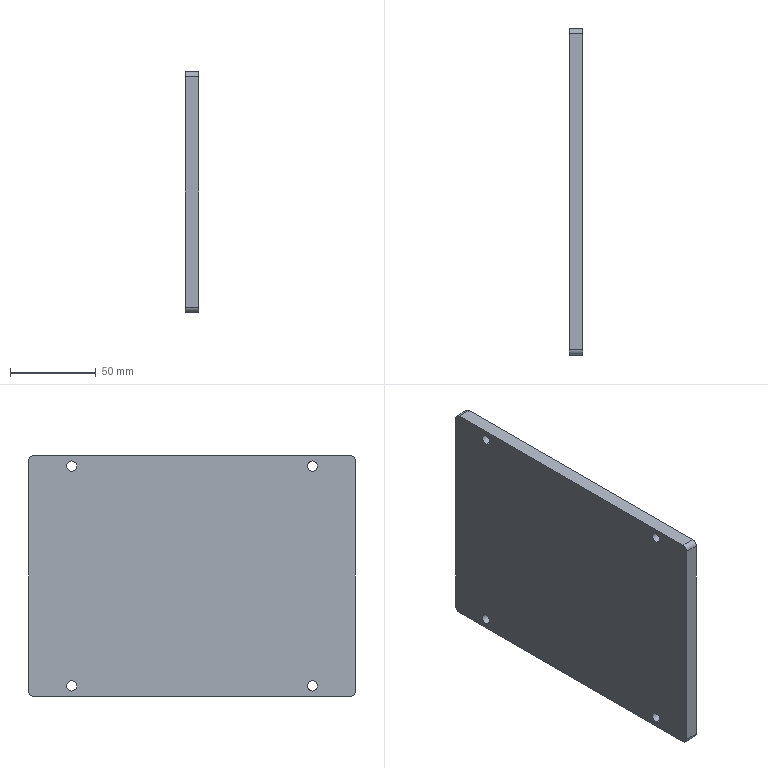Part | STEP file | RJWD-DY-B1_X2_5FEB5E7267DC680_2 | 1 solid | 18 faces | box 8 x 190 x 140 mm | volume 211833 mm3 | cylinder 12 | plane 6 | commonest cylinder face diameters 6 x12